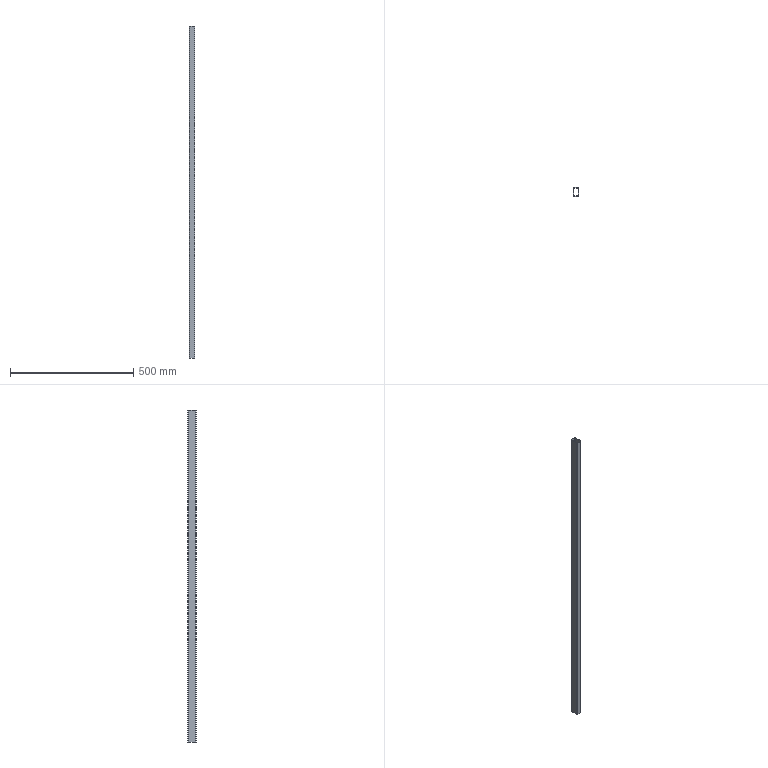Part | NX | 1 solid | 18 faces | box 24 x 36 x 1349 mm | volume 278141 mm3 | plane 10 | cylinder 8 | commonest cylinder face diameters 3.84 x4 7.68 x4
STEP:
#1=CARTESIAN_POINT('',(16.674,-653.339,607.953));
#2=VERTEX_POINT('',#1);
#3=CARTESIAN_POINT('',(12.834,-649.499,607.953));
#4=VERTEX_POINT('',#3);
#5=CARTESIAN_POINT('',(12.834,-653.339,607.953));
#6=DIRECTION('',(0.,0.,1.));
#7=DIRECTION('',(1.,0.,0.));
#8=AXIS2_PLACEMENT_3D('',#5,#6,#7);
#9=CIRCLE('',#8,3.84);
#10=EDGE_CURVE('',#2,#4,#9,.T.);
#11=ORIENTED_EDGE('',*,*,#10,.T.);
#12=CARTESIAN_POINT('',(12.834,-649.499,1957.099));
#13=VERTEX_POINT('',#12);
#14=CARTESIAN_POINT('',(12.834,-649.499,1957.099));
#15=DIRECTION('',(0.,0.,-1.));
#16=VECTOR('',#15,1.);
#17=LINE('',#14,#16);
#18=EDGE_CURVE('',#13,#4,#17,.T.);
#19=ORIENTED_EDGE('',*,*,#18,.F.);
#20=CARTESIAN_POINT('',(16.674,-653.339,1957.099));
#21=VERTEX_POINT('',#20);
#22=CARTESIAN_POINT('',(12.834,-653.339,1957.099));
#23=DIRECTION('',(0.,0.,1.));
#24=DIRECTION('',(1.,0.,0.));
#25=AXIS2_PLACEMENT_3D('',#22,#23,#24);
#26=CIRCLE('',#25,3.84);
#27=EDGE_CURVE('',#21,#13,#26,.T.);
#28=ORIENTED_EDGE('',*,*,#27,.F.);
#29=CARTESIAN_POINT('',(16.674,-653.339,1957.099));
#30=DIRECTION('',(0.,0.,-1.));
#31=VECTOR('',#30,1.);
#32=LINE('',#29,#31);
#33=EDGE_CURVE('',#21,#2,#32,.T.);
#34=ORIENTED_EDGE('',*,*,#33,.T.);
#35=EDGE_LOOP('',(#11,#19,#28,#34));
#36=FACE_OUTER_BOUND('',#35,.T.);
#37=CARTESIAN_POINT('',(12.834,-653.339,1957.099));
#38=DIRECTION('',(0.,0.,-1.));
#39=DIRECTION('',(0.,1.,0.));
#40=AXIS2_PLACEMENT_3D('',#37,#38,#39);
#41=CYLINDRICAL_SURFACE('',#40,3.84);
#42=ADVANCED_FACE('',(#36),#41,.T.);
#43=CARTESIAN_POINT('',(-3.486,-649.499,607.953));
#44=VERTEX_POINT('',#43);
#45=CARTESIAN_POINT('',(12.834,-649.499,607.953));
#46=DIRECTION('',(-1.,0.,0.));
#47=VECTOR('',#46,1.);
#48=LINE('',#45,#47);
#49=EDGE_CURVE('',#4,#44,#48,.T.);
#50=ORIENTED_EDGE('',*,*,#49,.T.);
#51=CARTESIAN_POINT('',(-3.486,-649.499,1957.099));
#52=VERTEX_POINT('',#51);
#53=CARTESIAN_POINT('',(-3.486,-649.499,1957.099));
#54=DIRECTION('',(0.,0.,-1.));
#55=VECTOR('',#54,1.);
#56=LINE('',#53,#55);
#57=EDGE_CURVE('',#52,#44,#56,.T.);
#58=ORIENTED_EDGE('',*,*,#57,.F.);
#59=CARTESIAN_POINT('',(12.834,-649.499,1957.099));
#60=DIRECTION('',(-1.,0.,0.));
#61=VECTOR('',#60,1.);
#62=LINE('',#59,#61);
#63=EDGE_CURVE('',#13,#52,#62,.T.);
#64=ORIENTED_EDGE('',*,*,#63,.F.);
#65=ORIENTED_EDGE('',*,*,#18,.T.);
#66=EDGE_LOOP('',(#50,#58,#64,#65));
#67=FACE_OUTER_BOUND('',#66,.T.);
#68=CARTESIAN_POINT('',(12.834,-649.499,1957.099));
#69=DIRECTION('',(0.,-1.,0.));
#70=DIRECTION('',(0.,0.,-1.));
#71=AXIS2_PLACEMENT_3D('',#68,#69,#70);
#72=PLANE('',#71);
#73=ADVANCED_FACE('',(#67),#72,.F.);
#74=CARTESIAN_POINT('',(-7.326,-653.339,607.953));
#75=VERTEX_POINT('',#74);
#76=CARTESIAN_POINT('',(-3.486,-653.339,607.953));
#77=DIRECTION('',(0.,0.,1.));
#78=DIRECTION('',(1.,0.,0.));
#79=AXIS2_PLACEMENT_3D('',#76,#77,#78);
#80=CIRCLE('',#79,3.84);
#81=EDGE_CURVE('',#44,#75,#80,.T.);
#82=ORIENTED_EDGE('',*,*,#81,.T.);
#83=CARTESIAN_POINT('',(-7.326,-653.339,1957.099));
#84=VERTEX_POINT('',#83);
#85=CARTESIAN_POINT('',(-7.326,-653.339,1957.099));
#86=DIRECTION('',(0.,0.,-1.));
#87=VECTOR('',#86,1.);
#88=LINE('',#85,#87);
#89=EDGE_CURVE('',#84,#75,#88,.T.);
#90=ORIENTED_EDGE('',*,*,#89,.F.);
#91=CARTESIAN_POINT('',(-3.486,-653.339,1957.099));
#92=DIRECTION('',(0.,0.,1.));
#93=DIRECTION('',(1.,0.,0.));
#94=AXIS2_PLACEMENT_3D('',#91,#92,#93);
#95=CIRCLE('',#94,3.84);
#96=EDGE_CURVE('',#52,#84,#95,.T.);
#97=ORIENTED_EDGE('',*,*,#96,.F.);
#98=ORIENTED_EDGE('',*,*,#57,.T.);
#99=EDGE_LOOP('',(#82,#90,#97,#98));
#100=FACE_OUTER_BOUND('',#99,.T.);
#101=CARTESIAN_POINT('',(-3.486,-653.339,1957.099));
#102=DIRECTION('',(0.,0.,-1.));
#103=DIRECTION('',(0.,1.,0.));
#104=AXIS2_PLACEMENT_3D('',#101,#102,#103);
#105=CYLINDRICAL_SURFACE('',#104,3.84);
#106=ADVANCED_FACE('',(#100),#105,.T.);
#107=CARTESIAN_POINT('',(-7.326,-681.659,607.953));
#108=VERTEX_POINT('',#107);
#109=CARTESIAN_POINT('',(-7.326,-681.659,607.953));
#110=DIRECTION('',(0.,-1.,0.));
#111=VECTOR('',#110,1.);
#112=LINE('',#109,#111);
#113=EDGE_CURVE('',#75,#108,#112,.T.);
#114=ORIENTED_EDGE('',*,*,#113,.T.);
#115=CARTESIAN_POINT('',(-7.326,-681.659,1957.099));
#116=VERTEX_POINT('',#115);
#117=CARTESIAN_POINT('',(-7.326,-681.659,1957.099));
#118=DIRECTION('',(0.,0.,-1.));
#119=VECTOR('',#118,1.);
#120=LINE('',#117,#119);
#121=EDGE_CURVE('',#116,#108,#120,.T.);
#122=ORIENTED_EDGE('',*,*,#121,.F.);
#123=CARTESIAN_POINT('',(-7.326,-681.659,1957.099));
#124=DIRECTION('',(0.,-1.,0.));
#125=VECTOR('',#124,1.);
#126=LINE('',#123,#125);
#127=EDGE_CURVE('',#84,#116,#126,.T.);
#128=ORIENTED_EDGE('',*,*,#127,.F.);
#129=ORIENTED_EDGE('',*,*,#89,.T.);
#130=EDGE_LOOP('',(#114,#122,#128,#129));
#131=FACE_OUTER_BOUND('',#130,.T.);
#132=CARTESIAN_POINT('',(-7.326,-681.659,1957.099));
#133=DIRECTION('',(1.,0.,0.));
#134=DIRECTION('',(0.,0.,-1.));
#135=AXIS2_PLACEMENT_3D('',#132,#133,#134);
#136=PLANE('',#135);
#137=ADVANCED_FACE('',(#131),#136,.F.);
#138=CARTESIAN_POINT('',(-3.486,-685.499,607.953));
#139=VERTEX_POINT('',#138);
#140=CARTESIAN_POINT('',(-3.486,-681.659,607.953));
#141=DIRECTION('',(0.,0.,1.));
#142=DIRECTION('',(1.,0.,0.));
#143=AXIS2_PLACEMENT_3D('',#140,#141,#142);
#144=CIRCLE('',#143,3.84);
#145=EDGE_CURVE('',#108,#139,#144,.T.);
#146=ORIENTED_EDGE('',*,*,#145,.T.);
#147=CARTESIAN_POINT('',(-3.486,-685.499,1957.099));
#148=VERTEX_POINT('',#147);
#149=CARTESIAN_POINT('',(-3.486,-685.499,1957.099));
#150=DIRECTION('',(0.,0.,-1.));
#151=VECTOR('',#150,1.);
#152=LINE('',#149,#151);
#153=EDGE_CURVE('',#148,#139,#152,.T.);
#154=ORIENTED_EDGE('',*,*,#153,.F.);
#155=CARTESIAN_POINT('',(-3.486,-681.659,1957.099));
#156=DIRECTION('',(0.,0.,1.));
#157=DIRECTION('',(1.,0.,0.));
#158=AXIS2_PLACEMENT_3D('',#155,#156,#157);
#159=CIRCLE('',#158,3.84);
#160=EDGE_CURVE('',#116,#148,#159,.T.);
#161=ORIENTED_EDGE('',*,*,#160,.F.);
#162=ORIENTED_EDGE('',*,*,#121,.T.);
#163=EDGE_LOOP('',(#146,#154,#161,#162));
#164=FACE_OUTER_BOUND('',#163,.T.);
#165=CARTESIAN_POINT('',(-3.486,-681.659,1957.099));
#166=DIRECTION('',(0.,0.,-1.));
#167=DIRECTION('',(0.,1.,0.));
#168=AXIS2_PLACEMENT_3D('',#165,#166,#167);
#169=CYLINDRICAL_SURFACE('',#168,3.84);
#170=ADVANCED_FACE('',(#164),#169,.T.);
#171=CARTESIAN_POINT('',(12.834,-685.499,607.953));
#172=VERTEX_POINT('',#171);
#173=CARTESIAN_POINT('',(-3.486,-685.499,607.953));
#174=DIRECTION('',(1.,0.,0.));
#175=VECTOR('',#174,1.);
#176=LINE('',#173,#175);
#177=EDGE_CURVE('',#139,#172,#176,.T.);
#178=ORIENTED_EDGE('',*,*,#177,.T.);
#179=CARTESIAN_POINT('',(12.834,-685.499,1957.099));
#180=VERTEX_POINT('',#179);
#181=CARTESIAN_POINT('',(12.834,-685.499,1957.099));
#182=DIRECTION('',(0.,0.,-1.));
#183=VECTOR('',#182,1.);
#184=LINE('',#181,#183);
#185=EDGE_CURVE('',#180,#172,#184,.T.);
#186=ORIENTED_EDGE('',*,*,#185,.F.);
#187=CARTESIAN_POINT('',(-3.486,-685.499,1957.099));
#188=DIRECTION('',(1.,0.,0.));
#189=VECTOR('',#188,1.);
#190=LINE('',#187,#189);
#191=EDGE_CURVE('',#148,#180,#190,.T.);
#192=ORIENTED_EDGE('',*,*,#191,.F.);
#193=ORIENTED_EDGE('',*,*,#153,.T.);
#194=EDGE_LOOP('',(#178,#186,#192,#193));
#195=FACE_OUTER_BOUND('',#194,.T.);
#196=CARTESIAN_POINT('',(-3.486,-685.499,1957.099));
#197=DIRECTION('',(0.,1.,0.));
#198=DIRECTION('',(0.,0.,1.));
#199=AXIS2_PLACEMENT_3D('',#196,#197,#198);
#200=PLANE('',#199);
#201=ADVANCED_FACE('',(#195),#200,.F.);
#202=CARTESIAN_POINT('',(16.674,-681.659,607.953));
#203=VERTEX_POINT('',#202);
#204=CARTESIAN_POINT('',(12.834,-681.659,607.953));
#205=DIRECTION('',(0.,0.,1.));
#206=DIRECTION('',(1.,0.,0.));
#207=AXIS2_PLACEMENT_3D('',#204,#205,#206);
#208=CIRCLE('',#207,3.84);
#209=EDGE_CURVE('',#172,#203,#208,.T.);
#210=ORIENTED_EDGE('',*,*,#209,.T.);
#211=CARTESIAN_POINT('',(16.674,-681.659,1957.099));
#212=VERTEX_POINT('',#211);
#213=CARTESIAN_POINT('',(16.674,-681.659,1957.099));
#214=DIRECTION('',(0.,0.,-1.));
#215=VECTOR('',#214,1.);
#216=LINE('',#213,#215);
#217=EDGE_CURVE('',#212,#203,#216,.T.);
#218=ORIENTED_EDGE('',*,*,#217,.F.);
#219=CARTESIAN_POINT('',(12.834,-681.659,1957.099));
#220=DIRECTION('',(0.,0.,1.));
#221=DIRECTION('',(1.,0.,0.));
#222=AXIS2_PLACEMENT_3D('',#219,#220,#221);
#223=CIRCLE('',#222,3.84);
#224=EDGE_CURVE('',#180,#212,#223,.T.);
#225=ORIENTED_EDGE('',*,*,#224,.F.);
#226=ORIENTED_EDGE('',*,*,#185,.T.);
#227=EDGE_LOOP('',(#210,#218,#225,#226));
#228=FACE_OUTER_BOUND('',#227,.T.);
#229=CARTESIAN_POINT('',(12.834,-681.659,1957.099));
#230=DIRECTION('',(0.,0.,-1.));
#231=DIRECTION('',(0.,1.,0.));
#232=AXIS2_PLACEMENT_3D('',#229,#230,#231);
#233=CYLINDRICAL_SURFACE('',#232,3.84);
#234=ADVANCED_FACE('',(#228),#233,.T.);
#235=CARTESIAN_POINT('',(-3.486,-651.419,607.953));
#236=VERTEX_POINT('',#235);
#237=CARTESIAN_POINT('',(-5.406,-653.339,607.953));
#238=VERTEX_POINT('',#237);
#239=CARTESIAN_POINT('',(-3.486,-653.339,607.953));
#240=DIRECTION('',(0.,0.,1.));
#241=DIRECTION('',(1.,0.,0.));
#242=AXIS2_PLACEMENT_3D('',#239,#240,#241);
#243=CIRCLE('',#242,1.92);
#244=EDGE_CURVE('',#236,#238,#243,.T.);
#245=ORIENTED_EDGE('',*,*,#244,.F.);
#246=CARTESIAN_POINT('',(-3.486,-651.419,1957.099));
#247=VERTEX_POINT('',#246);
#248=CARTESIAN_POINT('',(-3.486,-651.419,1957.099));
#249=DIRECTION('',(0.,0.,-1.));
#250=VECTOR('',#249,1.);
#251=LINE('',#248,#250);
#252=EDGE_CURVE('',#247,#236,#251,.T.);
#253=ORIENTED_EDGE('',*,*,#252,.F.);
#254=CARTESIAN_POINT('',(-5.406,-653.339,1957.099));
#255=VERTEX_POINT('',#254);
#256=CARTESIAN_POINT('',(-3.486,-653.339,1957.099));
#257=DIRECTION('',(0.,0.,1.));
#258=DIRECTION('',(1.,0.,0.));
#259=AXIS2_PLACEMENT_3D('',#256,#257,#258);
#260=CIRCLE('',#259,1.92);
#261=EDGE_CURVE('',#247,#255,#260,.T.);
#262=ORIENTED_EDGE('',*,*,#261,.T.);
#263=CARTESIAN_POINT('',(-5.406,-653.339,1957.099));
#264=DIRECTION('',(0.,0.,-1.));
#265=VECTOR('',#264,1.);
#266=LINE('',#263,#265);
#267=EDGE_CURVE('',#255,#238,#266,.T.);
#268=ORIENTED_EDGE('',*,*,#267,.T.);
#269=EDGE_LOOP('',(#245,#253,#262,#268));
#270=FACE_OUTER_BOUND('',#269,.T.);
#271=CARTESIAN_POINT('',(-3.486,-653.339,1957.099));
#272=DIRECTION('',(0.,0.,-1.));
#273=DIRECTION('',(0.,1.,0.));
#274=AXIS2_PLACEMENT_3D('',#271,#272,#273);
#275=CYLINDRICAL_SURFACE('',#274,1.92);
#276=ADVANCED_FACE('',(#270),#275,.F.);
#277=CARTESIAN_POINT('',(12.834,-651.419,607.953));
#278=VERTEX_POINT('',#277);
#279=CARTESIAN_POINT('',(12.834,-651.419,607.953));
#280=DIRECTION('',(-1.,0.,0.));
#281=VECTOR('',#280,1.);
#282=LINE('',#279,#281);
#283=EDGE_CURVE('',#278,#236,#282,.T.);
#284=ORIENTED_EDGE('',*,*,#283,.F.);
#285=CARTESIAN_POINT('',(12.834,-651.419,1957.099));
#286=VERTEX_POINT('',#285);
#287=CARTESIAN_POINT('',(12.834,-651.419,1957.099));
#288=DIRECTION('',(0.,0.,-1.));
#289=VECTOR('',#288,1.);
#290=LINE('',#287,#289);
#291=EDGE_CURVE('',#286,#278,#290,.T.);
#292=ORIENTED_EDGE('',*,*,#291,.F.);
#293=CARTESIAN_POINT('',(12.834,-651.419,1957.099));
#294=DIRECTION('',(-1.,0.,0.));
#295=VECTOR('',#294,1.);
#296=LINE('',#293,#295);
#297=EDGE_CURVE('',#286,#247,#296,.T.);
#298=ORIENTED_EDGE('',*,*,#297,.T.);
#299=ORIENTED_EDGE('',*,*,#252,.T.);
#300=EDGE_LOOP('',(#284,#292,#298,#299));
#301=FACE_OUTER_BOUND('',#300,.T.);
#302=CARTESIAN_POINT('',(12.834,-651.419,1957.099));
#303=DIRECTION('',(0.,-1.,0.));
#304=DIRECTION('',(0.,0.,-1.));
#305=AXIS2_PLACEMENT_3D('',#302,#303,#304);
#306=PLANE('',#305);
#307=ADVANCED_FACE('',(#301),#306,.T.);
#308=CARTESIAN_POINT('',(14.754,-653.339,607.953));
#309=VERTEX_POINT('',#308);
#310=CARTESIAN_POINT('',(12.834,-653.339,607.953));
#311=DIRECTION('',(0.,0.,1.));
#312=DIRECTION('',(1.,0.,0.));
#313=AXIS2_PLACEMENT_3D('',#310,#311,#312);
#314=CIRCLE('',#313,1.92);
#315=EDGE_CURVE('',#309,#278,#314,.T.);
#316=ORIENTED_EDGE('',*,*,#315,.F.);
#317=CARTESIAN_POINT('',(14.754,-653.339,1957.099));
#318=VERTEX_POINT('',#317);
#319=CARTESIAN_POINT('',(14.754,-653.339,1957.099));
#320=DIRECTION('',(0.,0.,-1.));
#321=VECTOR('',#320,1.);
#322=LINE('',#319,#321);
#323=EDGE_CURVE('',#318,#309,#322,.T.);
#324=ORIENTED_EDGE('',*,*,#323,.F.);
#325=CARTESIAN_POINT('',(12.834,-653.339,1957.099));
#326=DIRECTION('',(0.,0.,1.));
#327=DIRECTION('',(1.,0.,0.));
#328=AXIS2_PLACEMENT_3D('',#325,#326,#327);
#329=CIRCLE('',#328,1.92);
#330=EDGE_CURVE('',#318,#286,#329,.T.);
#331=ORIENTED_EDGE('',*,*,#330,.T.);
#332=ORIENTED_EDGE('',*,*,#291,.T.);
#333=EDGE_LOOP('',(#316,#324,#331,#332));
#334=FACE_OUTER_BOUND('',#333,.T.);
#335=CARTESIAN_POINT('',(12.834,-653.339,1957.099));
#336=DIRECTION('',(0.,0.,-1.));
#337=DIRECTION('',(0.,1.,0.));
#338=AXIS2_PLACEMENT_3D('',#335,#336,#337);
#339=CYLINDRICAL_SURFACE('',#338,1.92);
#340=ADVANCED_FACE('',(#334),#339,.F.);
#341=CARTESIAN_POINT('',(14.754,-681.659,607.953));
#342=VERTEX_POINT('',#341);
#343=CARTESIAN_POINT('',(14.754,-653.339,607.953));
#344=DIRECTION('',(0.,1.,0.));
#345=VECTOR('',#344,1.);
#346=LINE('',#343,#345);
#347=EDGE_CURVE('',#342,#309,#346,.T.);
#348=ORIENTED_EDGE('',*,*,#347,.F.);
#349=CARTESIAN_POINT('',(14.754,-681.659,1957.099));
#350=VERTEX_POINT('',#349);
#351=CARTESIAN_POINT('',(14.754,-681.659,1957.099));
#352=DIRECTION('',(0.,0.,-1.));
#353=VECTOR('',#352,1.);
#354=LINE('',#351,#353);
#355=EDGE_CURVE('',#350,#342,#354,.T.);
#356=ORIENTED_EDGE('',*,*,#355,.F.);
#357=CARTESIAN_POINT('',(14.754,-653.339,1957.099));
#358=DIRECTION('',(0.,1.,0.));
#359=VECTOR('',#358,1.);
#360=LINE('',#357,#359);
#361=EDGE_CURVE('',#350,#318,#360,.T.);
#362=ORIENTED_EDGE('',*,*,#361,.T.);
#363=ORIENTED_EDGE('',*,*,#323,.T.);
#364=EDGE_LOOP('',(#348,#356,#362,#363));
#365=FACE_OUTER_BOUND('',#364,.T.);
#366=CARTESIAN_POINT('',(14.754,-653.339,1957.099));
#367=DIRECTION('',(-1.,0.,0.));
#368=DIRECTION('',(0.,0.,1.));
#369=AXIS2_PLACEMENT_3D('',#366,#367,#368);
#370=PLANE('',#369);
#371=ADVANCED_FACE('',(#365),#370,.T.);
#372=CARTESIAN_POINT('',(12.834,-683.579,607.953));
#373=VERTEX_POINT('',#372);
#374=CARTESIAN_POINT('',(12.834,-681.659,607.953));
#375=DIRECTION('',(0.,0.,1.));
#376=DIRECTION('',(1.,0.,0.));
#377=AXIS2_PLACEMENT_3D('',#374,#375,#376);
#378=CIRCLE('',#377,1.92);
#379=EDGE_CURVE('',#373,#342,#378,.T.);
#380=ORIENTED_EDGE('',*,*,#379,.F.);
#381=CARTESIAN_POINT('',(12.834,-683.579,1957.099));
#382=VERTEX_POINT('',#381);
#383=CARTESIAN_POINT('',(12.834,-683.579,1957.099));
#384=DIRECTION('',(0.,0.,-1.));
#385=VECTOR('',#384,1.);
#386=LINE('',#383,#385);
#387=EDGE_CURVE('',#382,#373,#386,.T.);
#388=ORIENTED_EDGE('',*,*,#387,.F.);
#389=CARTESIAN_POINT('',(12.834,-681.659,1957.099));
#390=DIRECTION('',(0.,0.,1.));
#391=DIRECTION('',(1.,0.,0.));
#392=AXIS2_PLACEMENT_3D('',#389,#390,#391);
#393=CIRCLE('',#392,1.92);
#394=EDGE_CURVE('',#382,#350,#393,.T.);
#395=ORIENTED_EDGE('',*,*,#394,.T.);
#396=ORIENTED_EDGE('',*,*,#355,.T.);
#397=EDGE_LOOP('',(#380,#388,#395,#396));
#398=FACE_OUTER_BOUND('',#397,.T.);
#399=CARTESIAN_POINT('',(12.834,-681.659,1957.099));
#400=DIRECTION('',(0.,0.,-1.));
#401=DIRECTION('',(0.,1.,0.));
#402=AXIS2_PLACEMENT_3D('',#399,#400,#401);
#403=CYLINDRICAL_SURFACE('',#402,1.92);
#404=ADVANCED_FACE('',(#398),#403,.F.);
#405=CARTESIAN_POINT('',(-3.486,-683.579,607.953));
#406=VERTEX_POINT('',#405);
#407=CARTESIAN_POINT('',(-3.486,-683.579,607.953));
#408=DIRECTION('',(1.,0.,0.));
#409=VECTOR('',#408,1.);
#410=LINE('',#407,#409);
#411=EDGE_CURVE('',#406,#373,#410,.T.);
#412=ORIENTED_EDGE('',*,*,#411,.F.);
#413=CARTESIAN_POINT('',(-3.486,-683.579,1957.099));
#414=VERTEX_POINT('',#413);
#415=CARTESIAN_POINT('',(-3.486,-683.579,1957.099));
#416=DIRECTION('',(0.,0.,-1.));
#417=VECTOR('',#416,1.);
#418=LINE('',#415,#417);
#419=EDGE_CURVE('',#414,#406,#418,.T.);
#420=ORIENTED_EDGE('',*,*,#419,.F.);
#421=CARTESIAN_POINT('',(-3.486,-683.579,1957.099));
#422=DIRECTION('',(1.,0.,0.));
#423=VECTOR('',#422,1.);
#424=LINE('',#421,#423);
#425=EDGE_CURVE('',#414,#382,#424,.T.);
#426=ORIENTED_EDGE('',*,*,#425,.T.);
#427=ORIENTED_EDGE('',*,*,#387,.T.);
#428=EDGE_LOOP('',(#412,#420,#426,#427));
#429=FACE_OUTER_BOUND('',#428,.T.);
#430=CARTESIAN_POINT('',(-3.486,-683.579,1957.099));
#431=DIRECTION('',(0.,1.,0.));
#432=DIRECTION('',(0.,0.,1.));
#433=AXIS2_PLACEMENT_3D('',#430,#431,#432);
#434=PLANE('',#433);
#435=ADVANCED_FACE('',(#429),#434,.T.);
#436=CARTESIAN_POINT('',(-5.406,-681.659,607.953));
#437=VERTEX_POINT('',#436);
#438=CARTESIAN_POINT('',(-3.486,-681.659,607.953));
#439=DIRECTION('',(0.,0.,1.));
#440=DIRECTION('',(1.,0.,0.));
#441=AXIS2_PLACEMENT_3D('',#438,#439,#440);
#442=CIRCLE('',#441,1.92);
#443=EDGE_CURVE('',#437,#406,#442,.T.);
#444=ORIENTED_EDGE('',*,*,#443,.F.);
#445=CARTESIAN_POINT('',(-5.406,-681.659,1957.099));
#446=VERTEX_POINT('',#445);
#447=CARTESIAN_POINT('',(-5.406,-681.659,1957.099));
#448=DIRECTION('',(0.,0.,-1.));
#449=VECTOR('',#448,1.);
#450=LINE('',#447,#449);
#451=EDGE_CURVE('',#446,#437,#450,.T.);
#452=ORIENTED_EDGE('',*,*,#451,.F.);
#453=CARTESIAN_POINT('',(-3.486,-681.659,1957.099));
#454=DIRECTION('',(0.,0.,1.));
#455=DIRECTION('',(1.,0.,0.));
#456=AXIS2_PLACEMENT_3D('',#453,#454,#455);
#457=CIRCLE('',#456,1.92);
#458=EDGE_CURVE('',#446,#414,#457,.T.);
#459=ORIENTED_EDGE('',*,*,#458,.T.);
#460=ORIENTED_EDGE('',*,*,#419,.T.);
#461=EDGE_LOOP('',(#444,#452,#459,#460));
#462=FACE_OUTER_BOUND('',#461,.T.);
#463=CARTESIAN_POINT('',(-3.486,-681.659,1957.099));
#464=DIRECTION('',(0.,0.,-1.));
#465=DIRECTION('',(0.,1.,0.));
#466=AXIS2_PLACEMENT_3D('',#463,#464,#465);
#467=CYLINDRICAL_SURFACE('',#466,1.92);
#468=ADVANCED_FACE('',(#462),#467,.F.);
#469=CARTESIAN_POINT('',(-5.406,-681.659,607.953));
#470=DIRECTION('',(0.,-1.,0.));
#471=VECTOR('',#470,1.);
#472=LINE('',#469,#471);
#473=EDGE_CURVE('',#238,#437,#472,.T.);
#474=ORIENTED_EDGE('',*,*,#473,.F.);
#475=ORIENTED_EDGE('',*,*,#267,.F.);
#476=CARTESIAN_POINT('',(-5.406,-681.659,1957.099));
#477=DIRECTION('',(0.,-1.,0.));
#478=VECTOR('',#477,1.);
#479=LINE('',#476,#478);
#480=EDGE_CURVE('',#255,#446,#479,.T.);
#481=ORIENTED_EDGE('',*,*,#480,.T.);
#482=ORIENTED_EDGE('',*,*,#451,.T.);
#483=EDGE_LOOP('',(#474,#475,#481,#482));
#484=FACE_OUTER_BOUND('',#483,.T.);
#485=CARTESIAN_POINT('',(-5.406,-681.659,1957.099));
#486=DIRECTION('',(1.,0.,0.));
#487=DIRECTION('',(0.,0.,-1.));
#488=AXIS2_PLACEMENT_3D('',#485,#486,#487);
#489=PLANE('',#488);
#490=ADVANCED_FACE('',(#484),#489,.T.);
#491=CARTESIAN_POINT('',(16.674,-653.339,607.953));
#492=DIRECTION('',(0.,1.,0.));
#493=VECTOR('',#492,1.);
#494=LINE('',#491,#493);
#495=EDGE_CURVE('',#203,#2,#494,.T.);
#496=ORIENTED_EDGE('',*,*,#495,.T.);
#497=ORIENTED_EDGE('',*,*,#33,.F.);
#498=CARTESIAN_POINT('',(16.674,-653.339,1957.099));
#499=DIRECTION('',(0.,1.,0.));
#500=VECTOR('',#499,1.);
#501=LINE('',#498,#500);
#502=EDGE_CURVE('',#212,#21,#501,.T.);
#503=ORIENTED_EDGE('',*,*,#502,.F.);
#504=ORIENTED_EDGE('',*,*,#217,.T.);
#505=EDGE_LOOP('',(#496,#497,#503,#504));
#506=FACE_OUTER_BOUND('',#505,.T.);
#507=CARTESIAN_POINT('',(16.674,-653.339,1957.099));
#508=DIRECTION('',(-1.,0.,0.));
#509=DIRECTION('',(0.,0.,1.));
#510=AXIS2_PLACEMENT_3D('',#507,#508,#509);
#511=PLANE('',#510);
#512=ADVANCED_FACE('',(#506),#511,.F.);
#513=ORIENTED_EDGE('',*,*,#261,.F.);
#514=ORIENTED_EDGE('',*,*,#297,.F.);
#515=ORIENTED_EDGE('',*,*,#330,.F.);
#516=ORIENTED_EDGE('',*,*,#361,.F.);
#517=ORIENTED_EDGE('',*,*,#394,.F.);
#518=ORIENTED_EDGE('',*,*,#425,.F.);
#519=ORIENTED_EDGE('',*,*,#458,.F.);
#520=ORIENTED_EDGE('',*,*,#480,.F.);
#521=EDGE_LOOP('',(#513,#514,#515,#516,#517,#518,#519,#520));
#522=FACE_BOUND('',#521,.T.);
#523=ORIENTED_EDGE('',*,*,#27,.T.);
#524=ORIENTED_EDGE('',*,*,#63,.T.);
#525=ORIENTED_EDGE('',*,*,#96,.T.);
#526=ORIENTED_EDGE('',*,*,#127,.T.);
#527=ORIENTED_EDGE('',*,*,#160,.T.);
#528=ORIENTED_EDGE('',*,*,#191,.T.);
#529=ORIENTED_EDGE('',*,*,#224,.T.);
#530=ORIENTED_EDGE('',*,*,#502,.T.);
#531=EDGE_LOOP('',(#523,#524,#525,#526,#527,#528,#529,#530));
#532=FACE_BOUND('',#531,.T.);
#533=CARTESIAN_POINT('',(12.834,-653.339,1957.099));
#534=DIRECTION('',(0.,0.,1.));
#535=DIRECTION('',(1.,0.,0.));
#536=AXIS2_PLACEMENT_3D('',#533,#534,#535);
#537=PLANE('',#536);
#538=ADVANCED_FACE('',(#522,#532),#537,.T.);
#539=ORIENTED_EDGE('',*,*,#244,.T.);
#540=ORIENTED_EDGE('',*,*,#473,.T.);
#541=ORIENTED_EDGE('',*,*,#443,.T.);
#542=ORIENTED_EDGE('',*,*,#411,.T.);
#543=ORIENTED_EDGE('',*,*,#379,.T.);
#544=ORIENTED_EDGE('',*,*,#347,.T.);
#545=ORIENTED_EDGE('',*,*,#315,.T.);
#546=ORIENTED_EDGE('',*,*,#283,.T.);
#547=EDGE_LOOP('',(#539,#540,#541,#542,#543,#544,#545,#546));
#548=FACE_BOUND('',#547,.T.);
#549=ORIENTED_EDGE('',*,*,#10,.F.);
#550=ORIENTED_EDGE('',*,*,#495,.F.);
#551=ORIENTED_EDGE('',*,*,#209,.F.);
#552=ORIENTED_EDGE('',*,*,#177,.F.);
#553=ORIENTED_EDGE('',*,*,#145,.F.);
#554=ORIENTED_EDGE('',*,*,#113,.F.);
#555=ORIENTED_EDGE('',*,*,#81,.F.);
#556=ORIENTED_EDGE('',*,*,#49,.F.);
#557=EDGE_LOOP('',(#549,#550,#551,#552,#553,#554,#555,#556));
#558=FACE_BOUND('',#557,.T.);
#559=CARTESIAN_POINT('',(12.834,-653.339,607.953));
#560=DIRECTION('',(0.,0.,1.));
#561=DIRECTION('',(1.,0.,0.));
#562=AXIS2_PLACEMENT_3D('',#559,#560,#561);
#563=PLANE('',#562);
#564=ADVANCED_FACE('',(#548,#558),#563,.F.);
#565=CLOSED_SHELL('',(#42,#73,#106,#137,#170,#201,#234,#276,#307,#340,#371,#404,#435,#468,#490,#512,#538,#564));
#566=MANIFOLD_SOLID_BREP('',#565);
#567=(LENGTH_UNIT()NAMED_UNIT(*)SI_UNIT(.MILLI.,.METRE.));
#568=UNCERTAINTY_MEASURE_WITH_UNIT(LENGTH_MEASURE(0.00002),#567,'','');
#569=(NAMED_UNIT(*)PLANE_ANGLE_UNIT()SI_UNIT($,.RADIAN.));
#570=PLANE_ANGLE_MEASURE_WITH_UNIT(PLANE_ANGLE_MEASURE(0.01745),#569);
#571=DIMENSIONAL_EXPONENTS(0.,0.,0.,0.,0.,0.,0.);
#572=(CONVERSION_BASED_UNIT('DEGREE',#570)NAMED_UNIT(#571)PLANE_ANGLE_UNIT());
#573=(NAMED_UNIT(*)SI_UNIT($,.STERADIAN.)SOLID_ANGLE_UNIT());
#574=(GEOMETRIC_REPRESENTATION_CONTEXT(3)GLOBAL_UNCERTAINTY_ASSIGNED_CONTEXT((#568))GLOBAL_UNIT_ASSIGNED_CONTEXT((#567,#572,#573))REPRESENTATION_CONTEXT('',''));
#575=ADVANCED_BREP_SHAPE_REPRESENTATION('',(#566),#574);